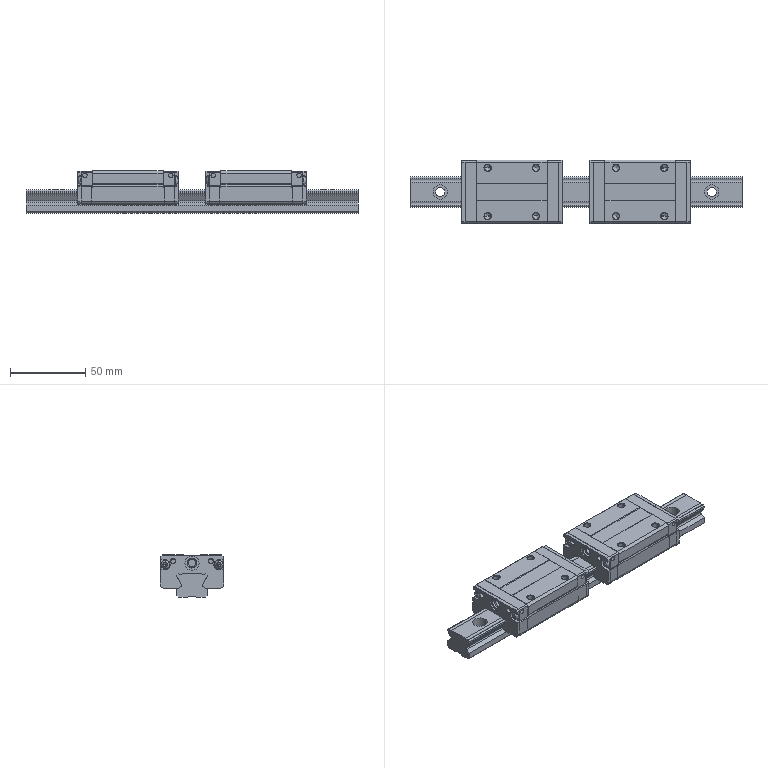Part | NX | 11 solids | 858 faces | box 220 x 42 x 28 mm | volume 139805 mm3 | plane 492 | cylinder 286 | cone 64 | torus 16 | commonest cylinder face diameters 3 x48 3.5 x32 6.5 x32 4 x20 1.51 x16 3.4 x16